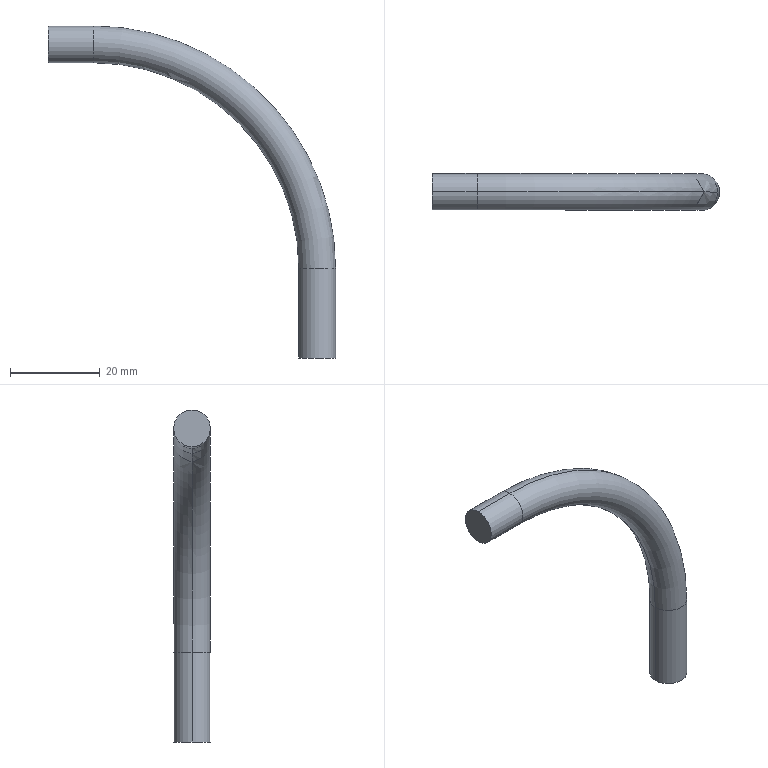Part | STEP file | ISPB-WXM-WA-750-10-650-T4-N-AQ-EB-G3-^-Part-5 | 1 solid | 8 faces | box 64.1 x 8.2 x 74.1 mm | volume 5732 mm3 | cylinder 4 | torus 2 | plane 2 | commonest cylinder face diameters 8.2 x4
STEP:
#1=CARTESIAN_POINT('',(0.,0.,0.));
#2=DIRECTION('',(0.,0.,1.));
#3=DIRECTION('',(1.,0.,0.));
#4=AXIS2_PLACEMENT_3D('',#1,#2,#3);
#5=CARTESIAN_POINT('',(361.5,14.,8.4));
#6=VERTEX_POINT('',#5);
#7=CARTESIAN_POINT('',(361.5,14.,0.2));
#8=VERTEX_POINT('',#7);
#9=CARTESIAN_POINT('',(361.5,14.,4.3));
#10=DIRECTION('',(-1.,0.,0.));
#11=DIRECTION('',(0.,0.,-1.));
#12=AXIS2_PLACEMENT_3D('',#9,#10,#11);
#13=CIRCLE('',#12,4.1);
#14=CARTESIAN_POINT('',(361.5,14.,-45.7));
#15=DIRECTION('',(0.,1.,0.));
#16=DIRECTION('',(-1.,0.,0.));
#17=AXIS2_PLACEMENT_3D('',#14,#15,#16);
#18=TOROIDAL_SURFACE('',#17,50.,4.1);
#19=CARTESIAN_POINT('',(1.571,-3.142));
#20=DIRECTION('',(0.,1.));
#21=VECTOR('',#20,1.);
#22=LINE('',#19,#21);
#23=(GEOMETRIC_REPRESENTATION_CONTEXT(2)PARAMETRIC_REPRESENTATION_CONTEXT()REPRESENTATION_CONTEXT('',''));
#24=DEFINITIONAL_REPRESENTATION('',(#22),#23);
#25=PCURVE('',#18,#24);
#26=CARTESIAN_POINT('',(361.5,14.,4.3));
#27=DIRECTION('',(-1.,0.,0.));
#28=DIRECTION('',(0.,0.,-1.));
#29=AXIS2_PLACEMENT_3D('',#26,#27,#28);
#30=CYLINDRICAL_SURFACE('',#29,4.1);
#31=CARTESIAN_POINT('',(0.,0.));
#32=DIRECTION('',(1.,0.));
#33=VECTOR('',#32,1.);
#34=LINE('',#31,#33);
#35=(GEOMETRIC_REPRESENTATION_CONTEXT(2)PARAMETRIC_REPRESENTATION_CONTEXT()REPRESENTATION_CONTEXT('',''));
#36=DEFINITIONAL_REPRESENTATION('',(#34),#35);
#37=PCURVE('',#30,#36);
#38=SURFACE_CURVE('',#13,(#25,#37),.PCURVE_S1.);
#39=EDGE_CURVE('',#6,#8,#38,.T.);
#40=ORIENTED_EDGE('',*,*,#39,.F.);
#41=CARTESIAN_POINT('',(415.6,14.,-45.7));
#42=VERTEX_POINT('',#41);
#43=CARTESIAN_POINT('',(361.5,14.,-45.7));
#44=DIRECTION('',(0.,1.,0.));
#45=DIRECTION('',(0.,0.,1.));
#46=AXIS2_PLACEMENT_3D('',#43,#44,#45);
#47=CIRCLE('',#46,54.1);
#48=CARTESIAN_POINT('',(1.571,0.));
#49=DIRECTION('',(1.,0.));
#50=VECTOR('',#49,1.);
#51=LINE('',#48,#50);
#52=(GEOMETRIC_REPRESENTATION_CONTEXT(2)PARAMETRIC_REPRESENTATION_CONTEXT()REPRESENTATION_CONTEXT('',''));
#53=DEFINITIONAL_REPRESENTATION('',(#51),#52);
#54=PCURVE('',#18,#53);
#55=CARTESIAN_POINT('',(361.5,14.,-45.7));
#56=DIRECTION('',(0.,1.,0.));
#57=DIRECTION('',(-1.,0.,0.));
#58=AXIS2_PLACEMENT_3D('',#55,#56,#57);
#59=TOROIDAL_SURFACE('',#58,50.,4.1);
#60=CARTESIAN_POINT('',(1.571,6.283));
#61=DIRECTION('',(1.,0.));
#62=VECTOR('',#61,1.);
#63=LINE('',#60,#62);
#64=(GEOMETRIC_REPRESENTATION_CONTEXT(2)PARAMETRIC_REPRESENTATION_CONTEXT()REPRESENTATION_CONTEXT('',''));
#65=DEFINITIONAL_REPRESENTATION('',(#63),#64);
#66=PCURVE('',#59,#65);
#67=SURFACE_CURVE('',#47,(#54,#66),.PCURVE_S1.);
#68=EDGE_CURVE('',#6,#42,#67,.T.);
#69=ORIENTED_EDGE('',*,*,#68,.T.);
#70=CARTESIAN_POINT('',(407.4,14.,-45.7));
#71=VERTEX_POINT('',#70);
#72=CARTESIAN_POINT('',(411.5,14.,-45.7));
#73=DIRECTION('',(0.,0.,-1.));
#74=DIRECTION('',(0.,1.,0.));
#75=AXIS2_PLACEMENT_3D('',#72,#73,#74);
#76=CIRCLE('',#75,4.1);
#77=CARTESIAN_POINT('',(3.142,7.854));
#78=DIRECTION('',(0.,-1.));
#79=VECTOR('',#78,1.);
#80=LINE('',#77,#79);
#81=(GEOMETRIC_REPRESENTATION_CONTEXT(2)PARAMETRIC_REPRESENTATION_CONTEXT()REPRESENTATION_CONTEXT('',''));
#82=DEFINITIONAL_REPRESENTATION('',(#80),#81);
#83=PCURVE('',#18,#82);
#84=CARTESIAN_POINT('',(411.5,14.,-45.7));
#85=DIRECTION('',(0.,0.,-1.));
#86=DIRECTION('',(1.,0.,0.));
#87=AXIS2_PLACEMENT_3D('',#84,#85,#86);
#88=CYLINDRICAL_SURFACE('',#87,4.1);
#89=CARTESIAN_POINT('',(-1.571,0.));
#90=DIRECTION('',(1.,0.));
#91=VECTOR('',#90,1.);
#92=LINE('',#89,#91);
#93=(GEOMETRIC_REPRESENTATION_CONTEXT(2)PARAMETRIC_REPRESENTATION_CONTEXT()REPRESENTATION_CONTEXT('',''));
#94=DEFINITIONAL_REPRESENTATION('',(#92),#93);
#95=PCURVE('',#88,#94);
#96=SURFACE_CURVE('',#76,(#83,#95),.PCURVE_S1.);
#97=EDGE_CURVE('',#71,#42,#96,.T.);
#98=ORIENTED_EDGE('',*,*,#97,.F.);
#99=CARTESIAN_POINT('',(361.5,14.,-45.7));
#100=DIRECTION('',(0.,1.,0.));
#101=DIRECTION('',(0.,0.,1.));
#102=AXIS2_PLACEMENT_3D('',#99,#100,#101);
#103=CIRCLE('',#102,45.9);
#104=CARTESIAN_POINT('',(1.571,3.142));
#105=DIRECTION('',(1.,0.));
#106=VECTOR('',#105,1.);
#107=LINE('',#104,#106);
#108=(GEOMETRIC_REPRESENTATION_CONTEXT(2)PARAMETRIC_REPRESENTATION_CONTEXT()REPRESENTATION_CONTEXT('',''));
#109=DEFINITIONAL_REPRESENTATION('',(#107),#108);
#110=PCURVE('',#18,#109);
#111=CARTESIAN_POINT('',(1.571,3.142));
#112=DIRECTION('',(1.,0.));
#113=VECTOR('',#112,1.);
#114=LINE('',#111,#113);
#115=(GEOMETRIC_REPRESENTATION_CONTEXT(2)PARAMETRIC_REPRESENTATION_CONTEXT()REPRESENTATION_CONTEXT('',''));
#116=DEFINITIONAL_REPRESENTATION('',(#114),#115);
#117=PCURVE('',#59,#116);
#118=SURFACE_CURVE('',#103,(#110,#117),.PCURVE_S1.);
#119=EDGE_CURVE('',#8,#71,#118,.T.);
#120=ORIENTED_EDGE('',*,*,#119,.F.);
#121=EDGE_LOOP('',(#40,#69,#98,#120));
#122=FACE_BOUND('',#121,.T.);
#123=ADVANCED_FACE('',(#122),#18,.T.);
#124=CARTESIAN_POINT('',(361.5,14.,4.3));
#125=DIRECTION('',(-1.,0.,0.));
#126=DIRECTION('',(0.,0.,-1.));
#127=AXIS2_PLACEMENT_3D('',#124,#125,#126);
#128=CIRCLE('',#127,4.1);
#129=CARTESIAN_POINT('',(361.5,14.,4.3));
#130=DIRECTION('',(-1.,0.,0.));
#131=DIRECTION('',(0.,0.,-1.));
#132=AXIS2_PLACEMENT_3D('',#129,#130,#131);
#133=CYLINDRICAL_SURFACE('',#132,4.1);
#134=CARTESIAN_POINT('',(0.,0.));
#135=DIRECTION('',(1.,0.));
#136=VECTOR('',#135,1.);
#137=LINE('',#134,#136);
#138=(GEOMETRIC_REPRESENTATION_CONTEXT(2)PARAMETRIC_REPRESENTATION_CONTEXT()REPRESENTATION_CONTEXT('',''));
#139=DEFINITIONAL_REPRESENTATION('',(#137),#138);
#140=PCURVE('',#133,#139);
#141=CARTESIAN_POINT('',(1.571,3.142));
#142=DIRECTION('',(0.,1.));
#143=VECTOR('',#142,1.);
#144=LINE('',#141,#143);
#145=(GEOMETRIC_REPRESENTATION_CONTEXT(2)PARAMETRIC_REPRESENTATION_CONTEXT()REPRESENTATION_CONTEXT('',''));
#146=DEFINITIONAL_REPRESENTATION('',(#144),#145);
#147=PCURVE('',#59,#146);
#148=SURFACE_CURVE('',#128,(#140,#147),.PCURVE_S1.);
#149=EDGE_CURVE('',#8,#6,#148,.T.);
#150=ORIENTED_EDGE('',*,*,#149,.T.);
#151=CARTESIAN_POINT('',(351.5,14.,8.4));
#152=VERTEX_POINT('',#151);
#153=CARTESIAN_POINT('',(361.5,14.,8.4));
#154=DIRECTION('',(-1.,0.,0.));
#155=VECTOR('',#154,1.);
#156=LINE('',#153,#155);
#157=CARTESIAN_POINT('',(3.142,0.));
#158=DIRECTION('',(0.,1.));
#159=VECTOR('',#158,1.);
#160=LINE('',#157,#159);
#161=(GEOMETRIC_REPRESENTATION_CONTEXT(2)PARAMETRIC_REPRESENTATION_CONTEXT()REPRESENTATION_CONTEXT('',''));
#162=DEFINITIONAL_REPRESENTATION('',(#160),#161);
#163=PCURVE('',#133,#162);
#164=CARTESIAN_POINT('',(3.142,0.));
#165=DIRECTION('',(0.,1.));
#166=VECTOR('',#165,1.);
#167=LINE('',#164,#166);
#168=(GEOMETRIC_REPRESENTATION_CONTEXT(2)PARAMETRIC_REPRESENTATION_CONTEXT()REPRESENTATION_CONTEXT('',''));
#169=DEFINITIONAL_REPRESENTATION('',(#167),#168);
#170=PCURVE('',#30,#169);
#171=SURFACE_CURVE('',#156,(#163,#170),.PCURVE_S1.);
#172=EDGE_CURVE('',#6,#152,#171,.T.);
#173=ORIENTED_EDGE('',*,*,#172,.T.);
#174=CARTESIAN_POINT('',(351.5,14.,0.2));
#175=VERTEX_POINT('',#174);
#176=CARTESIAN_POINT('',(351.5,14.,4.3));
#177=DIRECTION('',(1.,0.,0.));
#178=DIRECTION('',(0.,0.,1.));
#179=AXIS2_PLACEMENT_3D('',#176,#177,#178);
#180=CIRCLE('',#179,4.1);
#181=CARTESIAN_POINT('',(3.142,10.));
#182=DIRECTION('',(-1.,0.));
#183=VECTOR('',#182,1.);
#184=LINE('',#181,#183);
#185=(GEOMETRIC_REPRESENTATION_CONTEXT(2)PARAMETRIC_REPRESENTATION_CONTEXT()REPRESENTATION_CONTEXT('',''));
#186=DEFINITIONAL_REPRESENTATION('',(#184),#185);
#187=PCURVE('',#133,#186);
#188=CARTESIAN_POINT('',(351.5,14.,4.3));
#189=DIRECTION('',(-1.,0.,0.));
#190=DIRECTION('',(0.,0.,-1.));
#191=AXIS2_PLACEMENT_3D('',#188,#189,#190);
#192=PLANE('',#191);
#193=CARTESIAN_POINT('',(-4.1,0.));
#194=CARTESIAN_POINT('',(-4.1,7.101));
#195=CARTESIAN_POINT('',(2.05,3.551));
#196=CARTESIAN_POINT('',(8.2,0.));
#197=CARTESIAN_POINT('',(2.05,-3.551));
#198=CARTESIAN_POINT('',(-4.1,-7.101));
#199=CARTESIAN_POINT('',(-4.1,0.));
#200=(BOUNDED_CURVE()B_SPLINE_CURVE(2,(#193,#194,#195,#196,#197,#198,#199),.UNSPECIFIED.,.T.,.F.)B_SPLINE_CURVE_WITH_KNOTS((1,2,2,2,2,1),(-2.094,0.,2.094,4.189,6.283,8.378),.UNSPECIFIED.)CURVE()GEOMETRIC_REPRESENTATION_ITEM()RATIONAL_B_SPLINE_CURVE((1.,0.5,1.,0.5,1.,0.5,1.))REPRESENTATION_ITEM(''));
#201=(GEOMETRIC_REPRESENTATION_CONTEXT(2)PARAMETRIC_REPRESENTATION_CONTEXT()REPRESENTATION_CONTEXT('',''));
#202=DEFINITIONAL_REPRESENTATION('',(#200),#201);
#203=PCURVE('',#192,#202);
#204=SURFACE_CURVE('',#180,(#187,#203),.PCURVE_S1.);
#205=EDGE_CURVE('',#152,#175,#204,.T.);
#206=ORIENTED_EDGE('',*,*,#205,.T.);
#207=CARTESIAN_POINT('',(361.5,14.,0.2));
#208=DIRECTION('',(-1.,0.,0.));
#209=VECTOR('',#208,1.);
#210=LINE('',#207,#209);
#211=CARTESIAN_POINT('',(0.,0.));
#212=DIRECTION('',(0.,1.));
#213=VECTOR('',#212,1.);
#214=LINE('',#211,#213);
#215=(GEOMETRIC_REPRESENTATION_CONTEXT(2)PARAMETRIC_REPRESENTATION_CONTEXT()REPRESENTATION_CONTEXT('',''));
#216=DEFINITIONAL_REPRESENTATION('',(#214),#215);
#217=PCURVE('',#133,#216);
#218=CARTESIAN_POINT('',(6.283,0.));
#219=DIRECTION('',(0.,1.));
#220=VECTOR('',#219,1.);
#221=LINE('',#218,#220);
#222=(GEOMETRIC_REPRESENTATION_CONTEXT(2)PARAMETRIC_REPRESENTATION_CONTEXT()REPRESENTATION_CONTEXT('',''));
#223=DEFINITIONAL_REPRESENTATION('',(#221),#222);
#224=PCURVE('',#30,#223);
#225=SURFACE_CURVE('',#210,(#217,#224),.PCURVE_S1.);
#226=EDGE_CURVE('',#8,#175,#225,.T.);
#227=ORIENTED_EDGE('',*,*,#226,.F.);
#228=EDGE_LOOP('',(#150,#173,#206,#227));
#229=FACE_BOUND('',#228,.T.);
#230=ADVANCED_FACE('',(#229),#133,.T.);
#231=CARTESIAN_POINT('',(411.5,14.,-45.7));
#232=DIRECTION('',(0.,0.,-1.));
#233=DIRECTION('',(0.,1.,0.));
#234=AXIS2_PLACEMENT_3D('',#231,#232,#233);
#235=CIRCLE('',#234,4.1);
#236=CARTESIAN_POINT('',(411.5,14.,-45.7));
#237=DIRECTION('',(0.,0.,-1.));
#238=DIRECTION('',(1.,0.,0.));
#239=AXIS2_PLACEMENT_3D('',#236,#237,#238);
#240=CYLINDRICAL_SURFACE('',#239,4.1);
#241=CARTESIAN_POINT('',(-1.571,0.));
#242=DIRECTION('',(1.,0.));
#243=VECTOR('',#242,1.);
#244=LINE('',#241,#243);
#245=(GEOMETRIC_REPRESENTATION_CONTEXT(2)PARAMETRIC_REPRESENTATION_CONTEXT()REPRESENTATION_CONTEXT('',''));
#246=DEFINITIONAL_REPRESENTATION('',(#244),#245);
#247=PCURVE('',#240,#246);
#248=CARTESIAN_POINT('',(3.142,7.854));
#249=DIRECTION('',(0.,-1.));
#250=VECTOR('',#249,1.);
#251=LINE('',#248,#250);
#252=(GEOMETRIC_REPRESENTATION_CONTEXT(2)PARAMETRIC_REPRESENTATION_CONTEXT()REPRESENTATION_CONTEXT('',''));
#253=DEFINITIONAL_REPRESENTATION('',(#251),#252);
#254=PCURVE('',#59,#253);
#255=SURFACE_CURVE('',#235,(#247,#254),.PCURVE_S1.);
#256=EDGE_CURVE('',#42,#71,#255,.T.);
#257=ORIENTED_EDGE('',*,*,#256,.T.);
#258=CARTESIAN_POINT('',(407.4,14.,-65.7));
#259=VERTEX_POINT('',#258);
#260=CARTESIAN_POINT('',(407.4,14.,-45.7));
#261=DIRECTION('',(0.,0.,-1.));
#262=VECTOR('',#261,1.);
#263=LINE('',#260,#262);
#264=CARTESIAN_POINT('',(3.142,0.));
#265=DIRECTION('',(0.,1.));
#266=VECTOR('',#265,1.);
#267=LINE('',#264,#266);
#268=(GEOMETRIC_REPRESENTATION_CONTEXT(2)PARAMETRIC_REPRESENTATION_CONTEXT()REPRESENTATION_CONTEXT('',''));
#269=DEFINITIONAL_REPRESENTATION('',(#267),#268);
#270=PCURVE('',#240,#269);
#271=CARTESIAN_POINT('',(3.142,0.));
#272=DIRECTION('',(0.,1.));
#273=VECTOR('',#272,1.);
#274=LINE('',#271,#273);
#275=(GEOMETRIC_REPRESENTATION_CONTEXT(2)PARAMETRIC_REPRESENTATION_CONTEXT()REPRESENTATION_CONTEXT('',''));
#276=DEFINITIONAL_REPRESENTATION('',(#274),#275);
#277=PCURVE('',#88,#276);
#278=SURFACE_CURVE('',#263,(#270,#277),.PCURVE_S1.);
#279=EDGE_CURVE('',#71,#259,#278,.T.);
#280=ORIENTED_EDGE('',*,*,#279,.T.);
#281=CARTESIAN_POINT('',(415.6,14.,-65.7));
#282=VERTEX_POINT('',#281);
#283=CARTESIAN_POINT('',(411.5,14.,-65.7));
#284=DIRECTION('',(0.,0.,1.));
#285=DIRECTION('',(-1.,0.,0.));
#286=AXIS2_PLACEMENT_3D('',#283,#284,#285);
#287=CIRCLE('',#286,4.1);
#288=CARTESIAN_POINT('',(3.142,20.));
#289=DIRECTION('',(-1.,0.));
#290=VECTOR('',#289,1.);
#291=LINE('',#288,#290);
#292=(GEOMETRIC_REPRESENTATION_CONTEXT(2)PARAMETRIC_REPRESENTATION_CONTEXT()REPRESENTATION_CONTEXT('',''));
#293=DEFINITIONAL_REPRESENTATION('',(#291),#292);
#294=PCURVE('',#240,#293);
#295=CARTESIAN_POINT('',(411.5,14.,-65.7));
#296=DIRECTION('',(0.,0.,-1.));
#297=DIRECTION('',(1.,0.,0.));
#298=AXIS2_PLACEMENT_3D('',#295,#296,#297);
#299=PLANE('',#298);
#300=CARTESIAN_POINT('',(-4.1,0.));
#301=CARTESIAN_POINT('',(-4.1,7.101));
#302=CARTESIAN_POINT('',(2.05,3.551));
#303=CARTESIAN_POINT('',(8.2,0.));
#304=CARTESIAN_POINT('',(2.05,-3.551));
#305=CARTESIAN_POINT('',(-4.1,-7.101));
#306=CARTESIAN_POINT('',(-4.1,0.));
#307=(BOUNDED_CURVE()B_SPLINE_CURVE(2,(#300,#301,#302,#303,#304,#305,#306),.UNSPECIFIED.,.T.,.F.)B_SPLINE_CURVE_WITH_KNOTS((1,2,2,2,2,1),(-2.094,0.,2.094,4.189,6.283,8.378),.UNSPECIFIED.)CURVE()GEOMETRIC_REPRESENTATION_ITEM()RATIONAL_B_SPLINE_CURVE((1.,0.5,1.,0.5,1.,0.5,1.))REPRESENTATION_ITEM(''));
#308=(GEOMETRIC_REPRESENTATION_CONTEXT(2)PARAMETRIC_REPRESENTATION_CONTEXT()REPRESENTATION_CONTEXT('',''));
#309=DEFINITIONAL_REPRESENTATION('',(#307),#308);
#310=PCURVE('',#299,#309);
#311=SURFACE_CURVE('',#287,(#294,#310),.PCURVE_S1.);
#312=EDGE_CURVE('',#259,#282,#311,.T.);
#313=ORIENTED_EDGE('',*,*,#312,.T.);
#314=CARTESIAN_POINT('',(415.6,14.,-45.7));
#315=DIRECTION('',(0.,0.,-1.));
#316=VECTOR('',#315,1.);
#317=LINE('',#314,#316);
#318=CARTESIAN_POINT('',(0.,0.));
#319=DIRECTION('',(0.,1.));
#320=VECTOR('',#319,1.);
#321=LINE('',#318,#320);
#322=(GEOMETRIC_REPRESENTATION_CONTEXT(2)PARAMETRIC_REPRESENTATION_CONTEXT()REPRESENTATION_CONTEXT('',''));
#323=DEFINITIONAL_REPRESENTATION('',(#321),#322);
#324=PCURVE('',#240,#323);
#325=CARTESIAN_POINT('',(6.283,0.));
#326=DIRECTION('',(0.,1.));
#327=VECTOR('',#326,1.);
#328=LINE('',#325,#327);
#329=(GEOMETRIC_REPRESENTATION_CONTEXT(2)PARAMETRIC_REPRESENTATION_CONTEXT()REPRESENTATION_CONTEXT('',''));
#330=DEFINITIONAL_REPRESENTATION('',(#328),#329);
#331=PCURVE('',#88,#330);
#332=SURFACE_CURVE('',#317,(#324,#331),.PCURVE_S1.);
#333=EDGE_CURVE('',#42,#282,#332,.T.);
#334=ORIENTED_EDGE('',*,*,#333,.F.);
#335=EDGE_LOOP('',(#257,#280,#313,#334));
#336=FACE_BOUND('',#335,.T.);
#337=ADVANCED_FACE('',(#336),#240,.T.);
#338=ORIENTED_EDGE('',*,*,#68,.F.);
#339=ORIENTED_EDGE('',*,*,#149,.F.);
#340=ORIENTED_EDGE('',*,*,#119,.T.);
#341=ORIENTED_EDGE('',*,*,#256,.F.);
#342=EDGE_LOOP('',(#338,#339,#340,#341));
#343=FACE_BOUND('',#342,.T.);
#344=ADVANCED_FACE('',(#343),#59,.T.);
#345=CARTESIAN_POINT('',(411.5,14.,-65.7));
#346=DIRECTION('',(0.,0.,1.));
#347=DIRECTION('',(-1.,0.,0.));
#348=AXIS2_PLACEMENT_3D('',#345,#346,#347);
#349=CIRCLE('',#348,4.1);
#350=CARTESIAN_POINT('',(-4.1,0.));
#351=CARTESIAN_POINT('',(-4.1,7.101));
#352=CARTESIAN_POINT('',(2.05,3.551));
#353=CARTESIAN_POINT('',(8.2,0.));
#354=CARTESIAN_POINT('',(2.05,-3.551));
#355=CARTESIAN_POINT('',(-4.1,-7.101));
#356=CARTESIAN_POINT('',(-4.1,0.));
#357=(BOUNDED_CURVE()B_SPLINE_CURVE(2,(#350,#351,#352,#353,#354,#355,#356),.UNSPECIFIED.,.T.,.F.)B_SPLINE_CURVE_WITH_KNOTS((1,2,2,2,2,1),(-2.094,0.,2.094,4.189,6.283,8.378),.UNSPECIFIED.)CURVE()GEOMETRIC_REPRESENTATION_ITEM()RATIONAL_B_SPLINE_CURVE((1.,0.5,1.,0.5,1.,0.5,1.))REPRESENTATION_ITEM(''));
#358=(GEOMETRIC_REPRESENTATION_CONTEXT(2)PARAMETRIC_REPRESENTATION_CONTEXT()REPRESENTATION_CONTEXT('',''));
#359=DEFINITIONAL_REPRESENTATION('',(#357),#358);
#360=PCURVE('',#299,#359);
#361=CARTESIAN_POINT('',(9.425,20.));
#362=DIRECTION('',(-1.,0.));
#363=VECTOR('',#362,1.);
#364=LINE('',#361,#363);
#365=(GEOMETRIC_REPRESENTATION_CONTEXT(2)PARAMETRIC_REPRESENTATION_CONTEXT()REPRESENTATION_CONTEXT('',''));
#366=DEFINITIONAL_REPRESENTATION('',(#364),#365);
#367=PCURVE('',#88,#366);
#368=SURFACE_CURVE('',#349,(#360,#367),.PCURVE_S1.);
#369=EDGE_CURVE('',#282,#259,#368,.T.);
#370=ORIENTED_EDGE('',*,*,#369,.F.);
#371=ORIENTED_EDGE('',*,*,#312,.F.);
#372=EDGE_LOOP('',(#370,#371));
#373=FACE_BOUND('',#372,.T.);
#374=ADVANCED_FACE('',(#373),#299,.T.);
#375=ORIENTED_EDGE('',*,*,#279,.F.);
#376=ORIENTED_EDGE('',*,*,#97,.T.);
#377=ORIENTED_EDGE('',*,*,#333,.T.);
#378=ORIENTED_EDGE('',*,*,#369,.T.);
#379=EDGE_LOOP('',(#375,#376,#377,#378));
#380=FACE_BOUND('',#379,.T.);
#381=ADVANCED_FACE('',(#380),#88,.T.);
#382=CARTESIAN_POINT('',(351.5,14.,4.3));
#383=DIRECTION('',(1.,0.,0.));
#384=DIRECTION('',(0.,0.,1.));
#385=AXIS2_PLACEMENT_3D('',#382,#383,#384);
#386=CIRCLE('',#385,4.1);
#387=CARTESIAN_POINT('',(-4.1,0.));
#388=CARTESIAN_POINT('',(-4.1,7.101));
#389=CARTESIAN_POINT('',(2.05,3.551));
#390=CARTESIAN_POINT('',(8.2,0.));
#391=CARTESIAN_POINT('',(2.05,-3.551));
#392=CARTESIAN_POINT('',(-4.1,-7.101));
#393=CARTESIAN_POINT('',(-4.1,0.));
#394=(BOUNDED_CURVE()B_SPLINE_CURVE(2,(#387,#388,#389,#390,#391,#392,#393),.UNSPECIFIED.,.T.,.F.)B_SPLINE_CURVE_WITH_KNOTS((1,2,2,2,2,1),(-2.094,0.,2.094,4.189,6.283,8.378),.UNSPECIFIED.)CURVE()GEOMETRIC_REPRESENTATION_ITEM()RATIONAL_B_SPLINE_CURVE((1.,0.5,1.,0.5,1.,0.5,1.))REPRESENTATION_ITEM(''));
#395=(GEOMETRIC_REPRESENTATION_CONTEXT(2)PARAMETRIC_REPRESENTATION_CONTEXT()REPRESENTATION_CONTEXT('',''));
#396=DEFINITIONAL_REPRESENTATION('',(#394),#395);
#397=PCURVE('',#192,#396);
#398=CARTESIAN_POINT('',(9.425,10.));
#399=DIRECTION('',(-1.,0.));
#400=VECTOR('',#399,1.);
#401=LINE('',#398,#400);
#402=(GEOMETRIC_REPRESENTATION_CONTEXT(2)PARAMETRIC_REPRESENTATION_CONTEXT()REPRESENTATION_CONTEXT('',''));
#403=DEFINITIONAL_REPRESENTATION('',(#401),#402);
#404=PCURVE('',#30,#403);
#405=SURFACE_CURVE('',#386,(#397,#404),.PCURVE_S1.);
#406=EDGE_CURVE('',#175,#152,#405,.T.);
#407=ORIENTED_EDGE('',*,*,#406,.F.);
#408=ORIENTED_EDGE('',*,*,#205,.F.);
#409=EDGE_LOOP('',(#407,#408));
#410=FACE_BOUND('',#409,.T.);
#411=ADVANCED_FACE('',(#410),#192,.T.);
#412=ORIENTED_EDGE('',*,*,#172,.F.);
#413=ORIENTED_EDGE('',*,*,#39,.T.);
#414=ORIENTED_EDGE('',*,*,#226,.T.);
#415=ORIENTED_EDGE('',*,*,#406,.T.);
#416=EDGE_LOOP('',(#412,#413,#414,#415));
#417=FACE_BOUND('',#416,.T.);
#418=ADVANCED_FACE('',(#417),#30,.T.);
#419=CLOSED_SHELL('',(#123,#230,#337,#344,#374,#381,#411,#418));
#420=MANIFOLD_SOLID_BREP('',#419);
#421=(LENGTH_UNIT()NAMED_UNIT(*)SI_UNIT(.MILLI.,.METRE.));
#422=UNCERTAINTY_MEASURE_WITH_UNIT(LENGTH_MEASURE(0.0000001),#421,'','');
#423=(NAMED_UNIT(*)PLANE_ANGLE_UNIT()SI_UNIT($,.RADIAN.));
#424=(NAMED_UNIT(*)SI_UNIT($,.STERADIAN.)SOLID_ANGLE_UNIT());
#425=(GEOMETRIC_REPRESENTATION_CONTEXT(3)GLOBAL_UNCERTAINTY_ASSIGNED_CONTEXT((#422))GLOBAL_UNIT_ASSIGNED_CONTEXT((#421,#423,#424))REPRESENTATION_CONTEXT('',''));
#426=ADVANCED_BREP_SHAPE_REPRESENTATION('',(#4,#420),#425);